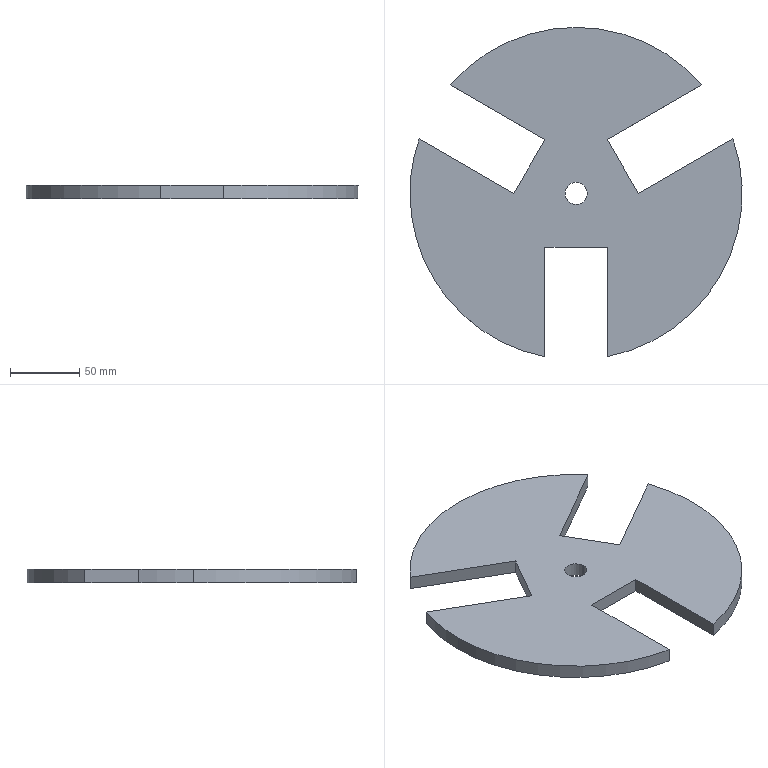Part | SolidWorks | features BaseBody 1 | 1 solid | 17 faces | box 240 x 237.872 x 10 mm | volume 341944 mm3 | plane 11 | cylinder 6 | commonest cylinder face diameters 240 x4 16 x2
STEP:
#1=CARTESIAN_POINT('',(298.547,1729.544,-1033.));
#2=VERTEX_POINT('',#1);
#3=CARTESIAN_POINT('',(282.547,1729.544,-1033.));
#4=VERTEX_POINT('',#3);
#5=CARTESIAN_POINT('',(290.547,1729.544,-1033.));
#6=DIRECTION('',(0.,0.,-1.));
#7=DIRECTION('',(1.,0.,0.));
#8=AXIS2_PLACEMENT_3D('',#5,#6,#7);
#9=CIRCLE('',#8,8.);
#10=EDGE_CURVE('',#2,#4,#9,.T.);
#11=ORIENTED_EDGE('',*,*,#10,.T.);
#12=CARTESIAN_POINT('',(282.547,1729.544,-1023.));
#13=VERTEX_POINT('',#12);
#14=CARTESIAN_POINT('',(282.547,1729.544,-1055.627));
#15=DIRECTION('',(0.,0.,1.));
#16=VECTOR('',#15,1000.);
#17=LINE('',#14,#16);
#18=EDGE_CURVE('',#4,#13,#17,.T.);
#19=ORIENTED_EDGE('',*,*,#18,.T.);
#20=CARTESIAN_POINT('',(298.547,1729.544,-1023.));
#21=VERTEX_POINT('',#20);
#22=CARTESIAN_POINT('',(290.547,1729.544,-1023.));
#23=DIRECTION('',(0.,0.,-1.));
#24=DIRECTION('',(1.,0.,0.));
#25=AXIS2_PLACEMENT_3D('',#22,#23,#24);
#26=CIRCLE('',#25,8.);
#27=EDGE_CURVE('',#21,#13,#26,.T.);
#28=ORIENTED_EDGE('',*,*,#27,.F.);
#29=CARTESIAN_POINT('',(298.547,1729.544,-1055.627));
#30=DIRECTION('',(0.,0.,1.));
#31=VECTOR('',#30,1000.);
#32=LINE('',#29,#31);
#33=EDGE_CURVE('',#2,#21,#32,.T.);
#34=ORIENTED_EDGE('',*,*,#33,.F.);
#35=EDGE_LOOP('',(#11,#19,#28,#34));
#36=FACE_OUTER_BOUND('',#35,.T.);
#37=CARTESIAN_POINT('',(290.547,1729.544,-1055.627));
#38=DIRECTION('',(0.,0.,1.));
#39=DIRECTION('',(1.,0.,0.));
#40=AXIS2_PLACEMENT_3D('',#37,#38,#39);
#41=CYLINDRICAL_SURFACE('',#40,8.);
#42=ADVANCED_FACE('',(#36),#41,.F.);
#43=CARTESIAN_POINT('',(268.047,1611.672,-1023.));
#44=VERTEX_POINT('',#43);
#45=CARTESIAN_POINT('',(170.547,1729.544,-1023.));
#46=VERTEX_POINT('',#45);
#47=CARTESIAN_POINT('',(290.547,1729.544,-1023.));
#48=DIRECTION('',(0.,0.,-1.));
#49=DIRECTION('',(-1.,0.,0.));
#50=AXIS2_PLACEMENT_3D('',#47,#48,#49);
#51=CIRCLE('',#50,120.);
#52=EDGE_CURVE('',#44,#46,#51,.T.);
#53=ORIENTED_EDGE('',*,*,#52,.T.);
#54=CARTESIAN_POINT('',(170.547,1729.544,-1033.));
#55=VERTEX_POINT('',#54);
#56=CARTESIAN_POINT('',(170.547,1729.544,-1023.));
#57=DIRECTION('',(0.,0.,-1.));
#58=VECTOR('',#57,1000.);
#59=LINE('',#56,#58);
#60=EDGE_CURVE('',#46,#55,#59,.T.);
#61=ORIENTED_EDGE('',*,*,#60,.T.);
#62=CARTESIAN_POINT('',(268.047,1611.672,-1033.));
#63=VERTEX_POINT('',#62);
#64=CARTESIAN_POINT('',(290.547,1729.544,-1033.));
#65=DIRECTION('',(0.,0.,1.));
#66=DIRECTION('',(-1.,0.,0.));
#67=AXIS2_PLACEMENT_3D('',#64,#65,#66);
#68=CIRCLE('',#67,120.);
#69=EDGE_CURVE('',#55,#63,#68,.T.);
#70=ORIENTED_EDGE('',*,*,#69,.T.);
#71=CARTESIAN_POINT('',(268.047,1611.672,-1023.));
#72=DIRECTION('',(0.,0.,1.));
#73=VECTOR('',#72,1000.);
#74=LINE('',#71,#73);
#75=EDGE_CURVE('',#63,#44,#74,.T.);
#76=ORIENTED_EDGE('',*,*,#75,.T.);
#77=EDGE_LOOP('',(#53,#61,#70,#76));
#78=FACE_OUTER_BOUND('',#77,.T.);
#79=CARTESIAN_POINT('',(290.547,1729.544,-1023.));
#80=DIRECTION('',(0.,0.,-1.));
#81=DIRECTION('',(-1.,0.,0.));
#82=AXIS2_PLACEMENT_3D('',#79,#80,#81);
#83=CYLINDRICAL_SURFACE('',#82,120.);
#84=ADVANCED_FACE('',(#78),#83,.T.);
#85=ORIENTED_EDGE('',*,*,#10,.F.);
#86=CARTESIAN_POINT('',(290.547,1729.544,-1033.));
#87=DIRECTION('',(0.,0.,-1.));
#88=DIRECTION('',(1.,0.,0.));
#89=AXIS2_PLACEMENT_3D('',#86,#87,#88);
#90=CIRCLE('',#89,8.);
#91=EDGE_CURVE('',#4,#2,#90,.T.);
#92=ORIENTED_EDGE('',*,*,#91,.F.);
#93=EDGE_LOOP('',(#85,#92));
#94=FACE_BOUND('',#93,.T.);
#95=CARTESIAN_POINT('',(177.217,1768.994,-1033.));
#96=VERTEX_POINT('',#95);
#97=CARTESIAN_POINT('',(290.547,1729.544,-1033.));
#98=DIRECTION('',(0.,0.,1.));
#99=DIRECTION('',(-1.,0.,0.));
#100=AXIS2_PLACEMENT_3D('',#97,#98,#99);
#101=CIRCLE('',#100,120.);
#102=EDGE_CURVE('',#96,#55,#101,.T.);
#103=ORIENTED_EDGE('',*,*,#102,.F.);
#104=CARTESIAN_POINT('',(245.547,1729.544,-1033.));
#105=VERTEX_POINT('',#104);
#106=CARTESIAN_POINT('',(245.547,1729.544,-1033.));
#107=DIRECTION('',(-0.866,0.5,0.));
#108=VECTOR('',#107,1000.);
#109=LINE('',#106,#108);
#110=EDGE_CURVE('',#105,#96,#109,.T.);
#111=ORIENTED_EDGE('',*,*,#110,.F.);
#112=CARTESIAN_POINT('',(268.047,1768.515,-1033.));
#113=VERTEX_POINT('',#112);
#114=CARTESIAN_POINT('',(268.047,1768.515,-1033.));
#115=DIRECTION('',(-0.5,-0.866,0.));
#116=VECTOR('',#115,1000.);
#117=LINE('',#114,#116);
#118=EDGE_CURVE('',#113,#105,#117,.T.);
#119=ORIENTED_EDGE('',*,*,#118,.F.);
#120=CARTESIAN_POINT('',(199.717,1807.965,-1033.));
#121=VERTEX_POINT('',#120);
#122=CARTESIAN_POINT('',(199.717,1807.965,-1033.));
#123=DIRECTION('',(0.866,-0.5,0.));
#124=VECTOR('',#123,1000.);
#125=LINE('',#122,#124);
#126=EDGE_CURVE('',#121,#113,#125,.T.);
#127=ORIENTED_EDGE('',*,*,#126,.F.);
#128=CARTESIAN_POINT('',(381.376,1807.965,-1033.));
#129=VERTEX_POINT('',#128);
#130=CARTESIAN_POINT('',(290.547,1729.544,-1033.));
#131=DIRECTION('',(0.,0.,1.));
#132=DIRECTION('',(-1.,0.,0.));
#133=AXIS2_PLACEMENT_3D('',#130,#131,#132);
#134=CIRCLE('',#133,120.);
#135=EDGE_CURVE('',#129,#121,#134,.T.);
#136=ORIENTED_EDGE('',*,*,#135,.F.);
#137=CARTESIAN_POINT('',(313.047,1768.515,-1033.));
#138=VERTEX_POINT('',#137);
#139=CARTESIAN_POINT('',(313.047,1768.515,-1033.));
#140=DIRECTION('',(0.866,0.5,0.));
#141=VECTOR('',#140,1000.);
#142=LINE('',#139,#141);
#143=EDGE_CURVE('',#138,#129,#142,.T.);
#144=ORIENTED_EDGE('',*,*,#143,.F.);
#145=CARTESIAN_POINT('',(335.547,1729.544,-1033.));
#146=VERTEX_POINT('',#145);
#147=CARTESIAN_POINT('',(335.547,1729.544,-1033.));
#148=DIRECTION('',(-0.5,0.866,0.));
#149=VECTOR('',#148,1000.);
#150=LINE('',#147,#149);
#151=EDGE_CURVE('',#146,#138,#150,.T.);
#152=ORIENTED_EDGE('',*,*,#151,.F.);
#153=CARTESIAN_POINT('',(403.876,1768.994,-1033.));
#154=VERTEX_POINT('',#153);
#155=CARTESIAN_POINT('',(403.876,1768.994,-1033.));
#156=DIRECTION('',(-0.866,-0.5,0.));
#157=VECTOR('',#156,1000.);
#158=LINE('',#155,#157);
#159=EDGE_CURVE('',#154,#146,#158,.T.);
#160=ORIENTED_EDGE('',*,*,#159,.F.);
#161=CARTESIAN_POINT('',(313.047,1611.672,-1033.));
#162=VERTEX_POINT('',#161);
#163=CARTESIAN_POINT('',(290.547,1729.544,-1033.));
#164=DIRECTION('',(0.,0.,1.));
#165=DIRECTION('',(-1.,0.,0.));
#166=AXIS2_PLACEMENT_3D('',#163,#164,#165);
#167=CIRCLE('',#166,120.);
#168=EDGE_CURVE('',#162,#154,#167,.T.);
#169=ORIENTED_EDGE('',*,*,#168,.F.);
#170=CARTESIAN_POINT('',(313.047,1690.573,-1033.));
#171=VERTEX_POINT('',#170);
#172=CARTESIAN_POINT('',(313.047,1729.544,-1033.));
#173=DIRECTION('',(0.,-1.,0.));
#174=VECTOR('',#173,1000.);
#175=LINE('',#172,#174);
#176=EDGE_CURVE('',#171,#162,#175,.T.);
#177=ORIENTED_EDGE('',*,*,#176,.F.);
#178=CARTESIAN_POINT('',(268.047,1690.573,-1033.));
#179=VERTEX_POINT('',#178);
#180=CARTESIAN_POINT('',(290.547,1690.573,-1033.));
#181=DIRECTION('',(1.,0.,0.));
#182=VECTOR('',#181,1000.);
#183=LINE('',#180,#182);
#184=EDGE_CURVE('',#179,#171,#183,.T.);
#185=ORIENTED_EDGE('',*,*,#184,.F.);
#186=CARTESIAN_POINT('',(268.047,1729.544,-1033.));
#187=DIRECTION('',(0.,1.,0.));
#188=VECTOR('',#187,1000.);
#189=LINE('',#186,#188);
#190=EDGE_CURVE('',#63,#179,#189,.T.);
#191=ORIENTED_EDGE('',*,*,#190,.F.);
#192=ORIENTED_EDGE('',*,*,#69,.F.);
#193=EDGE_LOOP('',(#103,#111,#119,#127,#136,#144,#152,#160,#169,#177,#185,#191,#192));
#194=FACE_OUTER_BOUND('',#193,.T.);
#195=CARTESIAN_POINT('',(290.547,1729.544,-1033.));
#196=DIRECTION('',(0.,0.,1.));
#197=DIRECTION('',(1.,0.,0.));
#198=AXIS2_PLACEMENT_3D('',#195,#196,#197);
#199=PLANE('',#198);
#200=ADVANCED_FACE('',(#94,#194),#199,.F.);
#201=ORIENTED_EDGE('',*,*,#18,.F.);
#202=ORIENTED_EDGE('',*,*,#91,.T.);
#203=ORIENTED_EDGE('',*,*,#33,.T.);
#204=CARTESIAN_POINT('',(290.547,1729.544,-1023.));
#205=DIRECTION('',(0.,0.,-1.));
#206=DIRECTION('',(1.,0.,0.));
#207=AXIS2_PLACEMENT_3D('',#204,#205,#206);
#208=CIRCLE('',#207,8.);
#209=EDGE_CURVE('',#13,#21,#208,.T.);
#210=ORIENTED_EDGE('',*,*,#209,.F.);
#211=EDGE_LOOP('',(#201,#202,#203,#210));
#212=FACE_OUTER_BOUND('',#211,.T.);
#213=CARTESIAN_POINT('',(290.547,1729.544,-1055.627));
#214=DIRECTION('',(0.,0.,1.));
#215=DIRECTION('',(1.,0.,0.));
#216=AXIS2_PLACEMENT_3D('',#213,#214,#215);
#217=CYLINDRICAL_SURFACE('',#216,8.);
#218=ADVANCED_FACE('',(#212),#217,.F.);
#219=CARTESIAN_POINT('',(268.047,1690.573,-1023.));
#220=VERTEX_POINT('',#219);
#221=CARTESIAN_POINT('',(268.047,1690.573,-1023.));
#222=DIRECTION('',(0.,1.,0.));
#223=VECTOR('',#222,1000.);
#224=LINE('',#221,#223);
#225=EDGE_CURVE('',#44,#220,#224,.T.);
#226=ORIENTED_EDGE('',*,*,#225,.F.);
#227=ORIENTED_EDGE('',*,*,#75,.F.);
#228=ORIENTED_EDGE('',*,*,#190,.T.);
#229=CARTESIAN_POINT('',(268.047,1690.573,-1023.));
#230=DIRECTION('',(0.,0.,-1.));
#231=VECTOR('',#230,1000.);
#232=LINE('',#229,#231);
#233=EDGE_CURVE('',#220,#179,#232,.T.);
#234=ORIENTED_EDGE('',*,*,#233,.F.);
#235=EDGE_LOOP('',(#226,#227,#228,#234));
#236=FACE_OUTER_BOUND('',#235,.T.);
#237=CARTESIAN_POINT('',(268.047,1690.573,-1023.));
#238=DIRECTION('',(-1.,0.,0.));
#239=DIRECTION('',(0.,0.,1.));
#240=AXIS2_PLACEMENT_3D('',#237,#238,#239);
#241=PLANE('',#240);
#242=ADVANCED_FACE('',(#236),#241,.F.);
#243=ORIENTED_EDGE('',*,*,#60,.F.);
#244=CARTESIAN_POINT('',(177.217,1768.994,-1023.));
#245=VERTEX_POINT('',#244);
#246=CARTESIAN_POINT('',(290.547,1729.544,-1023.));
#247=DIRECTION('',(0.,0.,-1.));
#248=DIRECTION('',(-1.,0.,0.));
#249=AXIS2_PLACEMENT_3D('',#246,#247,#248);
#250=CIRCLE('',#249,120.);
#251=EDGE_CURVE('',#46,#245,#250,.T.);
#252=ORIENTED_EDGE('',*,*,#251,.T.);
#253=CARTESIAN_POINT('',(177.217,1768.994,-1023.));
#254=DIRECTION('',(0.,0.,-1.));
#255=VECTOR('',#254,1000.);
#256=LINE('',#253,#255);
#257=EDGE_CURVE('',#245,#96,#256,.T.);
#258=ORIENTED_EDGE('',*,*,#257,.T.);
#259=ORIENTED_EDGE('',*,*,#102,.T.);
#260=EDGE_LOOP('',(#243,#252,#258,#259));
#261=FACE_OUTER_BOUND('',#260,.T.);
#262=CARTESIAN_POINT('',(290.547,1729.544,-1023.));
#263=DIRECTION('',(0.,0.,-1.));
#264=DIRECTION('',(-1.,0.,0.));
#265=AXIS2_PLACEMENT_3D('',#262,#263,#264);
#266=CYLINDRICAL_SURFACE('',#265,120.);
#267=ADVANCED_FACE('',(#261),#266,.T.);
#268=CARTESIAN_POINT('',(245.547,1729.544,-1023.));
#269=VERTEX_POINT('',#268);
#270=CARTESIAN_POINT('',(245.547,1729.544,-1023.));
#271=DIRECTION('',(-0.866,0.5,0.));
#272=VECTOR('',#271,1000.);
#273=LINE('',#270,#272);
#274=EDGE_CURVE('',#269,#245,#273,.T.);
#275=ORIENTED_EDGE('',*,*,#274,.F.);
#276=CARTESIAN_POINT('',(245.547,1729.544,-1023.));
#277=DIRECTION('',(0.,0.,1.));
#278=VECTOR('',#277,1000.);
#279=LINE('',#276,#278);
#280=EDGE_CURVE('',#105,#269,#279,.T.);
#281=ORIENTED_EDGE('',*,*,#280,.F.);
#282=ORIENTED_EDGE('',*,*,#110,.T.);
#283=ORIENTED_EDGE('',*,*,#257,.F.);
#284=EDGE_LOOP('',(#275,#281,#282,#283));
#285=FACE_OUTER_BOUND('',#284,.T.);
#286=CARTESIAN_POINT('',(245.547,1729.544,-1023.));
#287=DIRECTION('',(-0.5,-0.866,0.));
#288=DIRECTION('',(0.866,-0.5,0.));
#289=AXIS2_PLACEMENT_3D('',#286,#287,#288);
#290=PLANE('',#289);
#291=ADVANCED_FACE('',(#285),#290,.F.);
#292=CARTESIAN_POINT('',(268.047,1768.515,-1023.));
#293=VERTEX_POINT('',#292);
#294=CARTESIAN_POINT('',(245.547,1729.544,-1023.));
#295=DIRECTION('',(-0.5,-0.866,0.));
#296=VECTOR('',#295,1000.);
#297=LINE('',#294,#296);
#298=EDGE_CURVE('',#293,#269,#297,.T.);
#299=ORIENTED_EDGE('',*,*,#298,.F.);
#300=CARTESIAN_POINT('',(268.047,1768.515,-1023.));
#301=DIRECTION('',(0.,0.,1.));
#302=VECTOR('',#301,1000.);
#303=LINE('',#300,#302);
#304=EDGE_CURVE('',#113,#293,#303,.T.);
#305=ORIENTED_EDGE('',*,*,#304,.F.);
#306=ORIENTED_EDGE('',*,*,#118,.T.);
#307=ORIENTED_EDGE('',*,*,#280,.T.);
#308=EDGE_LOOP('',(#299,#305,#306,#307));
#309=FACE_OUTER_BOUND('',#308,.T.);
#310=CARTESIAN_POINT('',(245.547,1729.544,-1023.));
#311=DIRECTION('',(0.866,-0.5,0.));
#312=DIRECTION('',(0.5,0.866,0.));
#313=AXIS2_PLACEMENT_3D('',#310,#311,#312);
#314=PLANE('',#313);
#315=ADVANCED_FACE('',(#309),#314,.F.);
#316=CARTESIAN_POINT('',(199.717,1807.965,-1023.));
#317=VERTEX_POINT('',#316);
#318=CARTESIAN_POINT('',(268.047,1768.515,-1023.));
#319=DIRECTION('',(0.866,-0.5,0.));
#320=VECTOR('',#319,1000.);
#321=LINE('',#318,#320);
#322=EDGE_CURVE('',#317,#293,#321,.T.);
#323=ORIENTED_EDGE('',*,*,#322,.F.);
#324=CARTESIAN_POINT('',(199.717,1807.965,-1023.));
#325=DIRECTION('',(0.,0.,1.));
#326=VECTOR('',#325,1000.);
#327=LINE('',#324,#326);
#328=EDGE_CURVE('',#121,#317,#327,.T.);
#329=ORIENTED_EDGE('',*,*,#328,.F.);
#330=ORIENTED_EDGE('',*,*,#126,.T.);
#331=ORIENTED_EDGE('',*,*,#304,.T.);
#332=EDGE_LOOP('',(#323,#329,#330,#331));
#333=FACE_OUTER_BOUND('',#332,.T.);
#334=CARTESIAN_POINT('',(268.047,1768.515,-1023.));
#335=DIRECTION('',(0.5,0.866,0.));
#336=DIRECTION('',(-0.866,0.5,0.));
#337=AXIS2_PLACEMENT_3D('',#334,#335,#336);
#338=PLANE('',#337);
#339=ADVANCED_FACE('',(#333),#338,.F.);
#340=CARTESIAN_POINT('',(381.376,1807.965,-1023.));
#341=VERTEX_POINT('',#340);
#342=CARTESIAN_POINT('',(381.376,1807.965,-1023.));
#343=DIRECTION('',(0.,0.,-1.));
#344=VECTOR('',#343,1000.);
#345=LINE('',#342,#344);
#346=EDGE_CURVE('',#341,#129,#345,.T.);
#347=ORIENTED_EDGE('',*,*,#346,.T.);
#348=ORIENTED_EDGE('',*,*,#135,.T.);
#349=ORIENTED_EDGE('',*,*,#328,.T.);
#350=CARTESIAN_POINT('',(290.547,1729.544,-1023.));
#351=DIRECTION('',(0.,0.,-1.));
#352=DIRECTION('',(-1.,0.,0.));
#353=AXIS2_PLACEMENT_3D('',#350,#351,#352);
#354=CIRCLE('',#353,120.);
#355=EDGE_CURVE('',#317,#341,#354,.T.);
#356=ORIENTED_EDGE('',*,*,#355,.T.);
#357=EDGE_LOOP('',(#347,#348,#349,#356));
#358=FACE_OUTER_BOUND('',#357,.T.);
#359=CARTESIAN_POINT('',(290.547,1729.544,-1023.));
#360=DIRECTION('',(0.,0.,-1.));
#361=DIRECTION('',(-1.,0.,0.));
#362=AXIS2_PLACEMENT_3D('',#359,#360,#361);
#363=CYLINDRICAL_SURFACE('',#362,120.);
#364=ADVANCED_FACE('',(#358),#363,.T.);
#365=CARTESIAN_POINT('',(313.047,1768.515,-1023.));
#366=VERTEX_POINT('',#365);
#367=CARTESIAN_POINT('',(313.047,1768.515,-1023.));
#368=DIRECTION('',(0.866,0.5,0.));
#369=VECTOR('',#368,1000.);
#370=LINE('',#367,#369);
#371=EDGE_CURVE('',#366,#341,#370,.T.);
#372=ORIENTED_EDGE('',*,*,#371,.F.);
#373=CARTESIAN_POINT('',(313.047,1768.515,-1023.));
#374=DIRECTION('',(0.,0.,1.));
#375=VECTOR('',#374,1000.);
#376=LINE('',#373,#375);
#377=EDGE_CURVE('',#138,#366,#376,.T.);
#378=ORIENTED_EDGE('',*,*,#377,.F.);
#379=ORIENTED_EDGE('',*,*,#143,.T.);
#380=ORIENTED_EDGE('',*,*,#346,.F.);
#381=EDGE_LOOP('',(#372,#378,#379,#380));
#382=FACE_OUTER_BOUND('',#381,.T.);
#383=CARTESIAN_POINT('',(313.047,1768.515,-1023.));
#384=DIRECTION('',(-0.5,0.866,0.));
#385=DIRECTION('',(-0.866,-0.5,0.));
#386=AXIS2_PLACEMENT_3D('',#383,#384,#385);
#387=PLANE('',#386);
#388=ADVANCED_FACE('',(#382),#387,.F.);
#389=CARTESIAN_POINT('',(335.547,1729.544,-1023.));
#390=VERTEX_POINT('',#389);
#391=CARTESIAN_POINT('',(335.547,1729.544,-1023.));
#392=DIRECTION('',(-0.5,0.866,0.));
#393=VECTOR('',#392,1000.);
#394=LINE('',#391,#393);
#395=EDGE_CURVE('',#390,#366,#394,.T.);
#396=ORIENTED_EDGE('',*,*,#395,.F.);
#397=CARTESIAN_POINT('',(335.547,1729.544,-1023.));
#398=DIRECTION('',(0.,0.,1.));
#399=VECTOR('',#398,1000.);
#400=LINE('',#397,#399);
#401=EDGE_CURVE('',#146,#390,#400,.T.);
#402=ORIENTED_EDGE('',*,*,#401,.F.);
#403=ORIENTED_EDGE('',*,*,#151,.T.);
#404=ORIENTED_EDGE('',*,*,#377,.T.);
#405=EDGE_LOOP('',(#396,#402,#403,#404));
#406=FACE_OUTER_BOUND('',#405,.T.);
#407=CARTESIAN_POINT('',(335.547,1729.544,-1023.));
#408=DIRECTION('',(-0.866,-0.5,0.));
#409=DIRECTION('',(0.5,-0.866,0.));
#410=AXIS2_PLACEMENT_3D('',#407,#408,#409);
#411=PLANE('',#410);
#412=ADVANCED_FACE('',(#406),#411,.F.);
#413=CARTESIAN_POINT('',(403.876,1768.994,-1023.));
#414=VERTEX_POINT('',#413);
#415=CARTESIAN_POINT('',(335.547,1729.544,-1023.));
#416=DIRECTION('',(-0.866,-0.5,0.));
#417=VECTOR('',#416,1000.);
#418=LINE('',#415,#417);
#419=EDGE_CURVE('',#414,#390,#418,.T.);
#420=ORIENTED_EDGE('',*,*,#419,.F.);
#421=CARTESIAN_POINT('',(403.876,1768.994,-1023.));
#422=DIRECTION('',(0.,0.,1.));
#423=VECTOR('',#422,1000.);
#424=LINE('',#421,#423);
#425=EDGE_CURVE('',#154,#414,#424,.T.);
#426=ORIENTED_EDGE('',*,*,#425,.F.);
#427=ORIENTED_EDGE('',*,*,#159,.T.);
#428=ORIENTED_EDGE('',*,*,#401,.T.);
#429=EDGE_LOOP('',(#420,#426,#427,#428));
#430=FACE_OUTER_BOUND('',#429,.T.);
#431=CARTESIAN_POINT('',(335.547,1729.544,-1023.));
#432=DIRECTION('',(0.5,-0.866,0.));
#433=DIRECTION('',(0.866,0.5,0.));
#434=AXIS2_PLACEMENT_3D('',#431,#432,#433);
#435=PLANE('',#434);
#436=ADVANCED_FACE('',(#430),#435,.F.);
#437=CARTESIAN_POINT('',(313.047,1611.672,-1023.));
#438=VERTEX_POINT('',#437);
#439=CARTESIAN_POINT('',(313.047,1611.672,-1023.));
#440=DIRECTION('',(0.,0.,-1.));
#441=VECTOR('',#440,1000.);
#442=LINE('',#439,#441);
#443=EDGE_CURVE('',#438,#162,#442,.T.);
#444=ORIENTED_EDGE('',*,*,#443,.T.);
#445=ORIENTED_EDGE('',*,*,#168,.T.);
#446=ORIENTED_EDGE('',*,*,#425,.T.);
#447=CARTESIAN_POINT('',(290.547,1729.544,-1023.));
#448=DIRECTION('',(0.,0.,-1.));
#449=DIRECTION('',(-1.,0.,0.));
#450=AXIS2_PLACEMENT_3D('',#447,#448,#449);
#451=CIRCLE('',#450,120.);
#452=EDGE_CURVE('',#414,#438,#451,.T.);
#453=ORIENTED_EDGE('',*,*,#452,.T.);
#454=EDGE_LOOP('',(#444,#445,#446,#453));
#455=FACE_OUTER_BOUND('',#454,.T.);
#456=CARTESIAN_POINT('',(290.547,1729.544,-1023.));
#457=DIRECTION('',(0.,0.,-1.));
#458=DIRECTION('',(-1.,0.,0.));
#459=AXIS2_PLACEMENT_3D('',#456,#457,#458);
#460=CYLINDRICAL_SURFACE('',#459,120.);
#461=ADVANCED_FACE('',(#455),#460,.T.);
#462=CARTESIAN_POINT('',(313.047,1690.573,-1023.));
#463=VERTEX_POINT('',#462);
#464=CARTESIAN_POINT('',(313.047,1690.573,-1023.));
#465=DIRECTION('',(0.,-1.,0.));
#466=VECTOR('',#465,1000.);
#467=LINE('',#464,#466);
#468=EDGE_CURVE('',#463,#438,#467,.T.);
#469=ORIENTED_EDGE('',*,*,#468,.F.);
#470=CARTESIAN_POINT('',(313.047,1690.573,-1023.));
#471=DIRECTION('',(0.,0.,1.));
#472=VECTOR('',#471,1000.);
#473=LINE('',#470,#472);
#474=EDGE_CURVE('',#171,#463,#473,.T.);
#475=ORIENTED_EDGE('',*,*,#474,.F.);
#476=ORIENTED_EDGE('',*,*,#176,.T.);
#477=ORIENTED_EDGE('',*,*,#443,.F.);
#478=EDGE_LOOP('',(#469,#475,#476,#477));
#479=FACE_OUTER_BOUND('',#478,.T.);
#480=CARTESIAN_POINT('',(313.047,1690.573,-1023.));
#481=DIRECTION('',(1.,0.,0.));
#482=DIRECTION('',(0.,0.,-1.));
#483=AXIS2_PLACEMENT_3D('',#480,#481,#482);
#484=PLANE('',#483);
#485=ADVANCED_FACE('',(#479),#484,.F.);
#486=CARTESIAN_POINT('',(313.047,1690.573,-1023.));
#487=DIRECTION('',(1.,0.,0.));
#488=VECTOR('',#487,1000.);
#489=LINE('',#486,#488);
#490=EDGE_CURVE('',#220,#463,#489,.T.);
#491=ORIENTED_EDGE('',*,*,#490,.F.);
#492=ORIENTED_EDGE('',*,*,#233,.T.);
#493=ORIENTED_EDGE('',*,*,#184,.T.);
#494=ORIENTED_EDGE('',*,*,#474,.T.);
#495=EDGE_LOOP('',(#491,#492,#493,#494));
#496=FACE_OUTER_BOUND('',#495,.T.);
#497=CARTESIAN_POINT('',(313.047,1690.573,-1023.));
#498=DIRECTION('',(0.,1.,0.));
#499=DIRECTION('',(0.,0.,1.));
#500=AXIS2_PLACEMENT_3D('',#497,#498,#499);
#501=PLANE('',#500);
#502=ADVANCED_FACE('',(#496),#501,.F.);
#503=ORIENTED_EDGE('',*,*,#27,.T.);
#504=ORIENTED_EDGE('',*,*,#209,.T.);
#505=EDGE_LOOP('',(#503,#504));
#506=FACE_BOUND('',#505,.T.);
#507=ORIENTED_EDGE('',*,*,#225,.T.);
#508=ORIENTED_EDGE('',*,*,#490,.T.);
#509=ORIENTED_EDGE('',*,*,#468,.T.);
#510=ORIENTED_EDGE('',*,*,#452,.F.);
#511=ORIENTED_EDGE('',*,*,#419,.T.);
#512=ORIENTED_EDGE('',*,*,#395,.T.);
#513=ORIENTED_EDGE('',*,*,#371,.T.);
#514=ORIENTED_EDGE('',*,*,#355,.F.);
#515=ORIENTED_EDGE('',*,*,#322,.T.);
#516=ORIENTED_EDGE('',*,*,#298,.T.);
#517=ORIENTED_EDGE('',*,*,#274,.T.);
#518=ORIENTED_EDGE('',*,*,#251,.F.);
#519=ORIENTED_EDGE('',*,*,#52,.F.);
#520=EDGE_LOOP('',(#507,#508,#509,#510,#511,#512,#513,#514,#515,#516,#517,#518,#519));
#521=FACE_OUTER_BOUND('',#520,.T.);
#522=CARTESIAN_POINT('',(290.547,1729.544,-1023.));
#523=DIRECTION('',(0.,0.,1.));
#524=DIRECTION('',(1.,0.,0.));
#525=AXIS2_PLACEMENT_3D('',#522,#523,#524);
#526=PLANE('',#525);
#527=ADVANCED_FACE('',(#506,#521),#526,.T.);
#528=CLOSED_SHELL('',(#42,#84,#200,#218,#242,#267,#291,#315,#339,#364,#388,#412,#436,#461,#485,#502,#527));
#529=MANIFOLD_SOLID_BREP('',#528);
#530=CARTESIAN_POINT('',(0.,0.,0.));
#531=DIRECTION('',(0.,0.,1.));
#532=DIRECTION('',(1.,0.,0.));
#533=AXIS2_PLACEMENT_3D('',#530,#531,#532);
#534=(LENGTH_UNIT()NAMED_UNIT(*)SI_UNIT(.MILLI.,.METRE.));
#535=UNCERTAINTY_MEASURE_WITH_UNIT(LENGTH_MEASURE(0.00001),#534,'','');
#536=(NAMED_UNIT(*)PLANE_ANGLE_UNIT()SI_UNIT($,.RADIAN.));
#537=(NAMED_UNIT(*)SI_UNIT($,.STERADIAN.)SOLID_ANGLE_UNIT());
#538=(GEOMETRIC_REPRESENTATION_CONTEXT(3)GLOBAL_UNCERTAINTY_ASSIGNED_CONTEXT((#535))GLOBAL_UNIT_ASSIGNED_CONTEXT((#534,#536,#537))REPRESENTATION_CONTEXT('',''));
#539=ADVANCED_BREP_SHAPE_REPRESENTATION('',(#529,#533),#538);